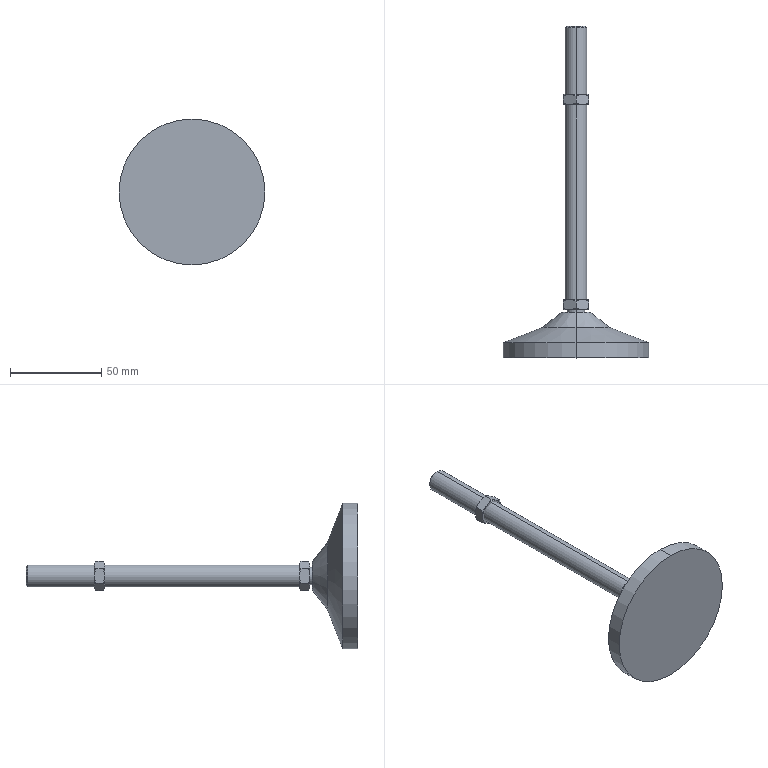Part | SolidWorks | features ICE 6, Chamfer 1, Revolution 1 | 3 solids | 60 faces | box 80 x 182 x 80 mm | volume 89449 mm3 | cone 34 | plane 20 | cylinder 6 | commonest cylinder face diameters 9.6 x2 12 x2 80 x2